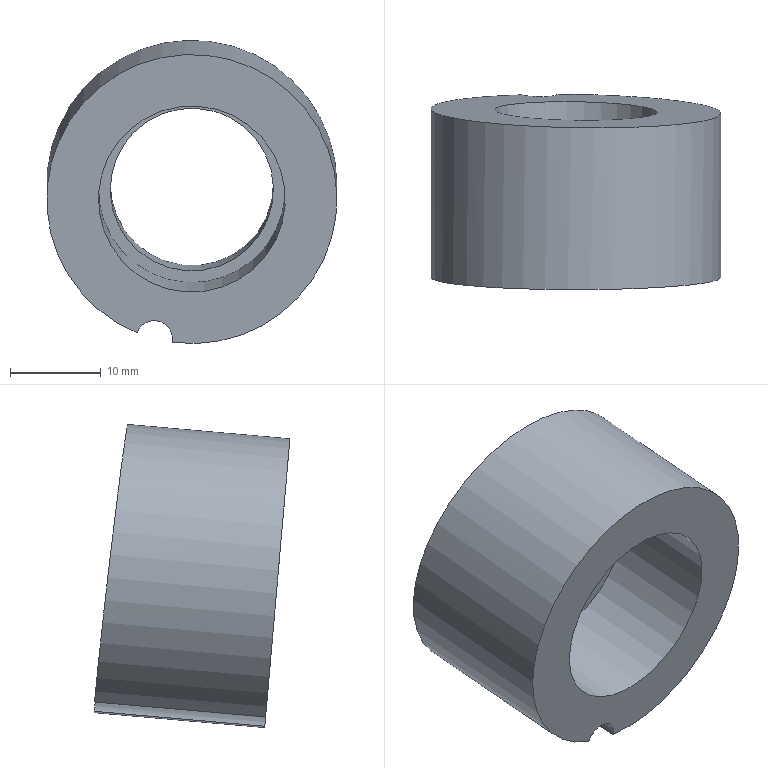Part | NX | features EKSD 32-20-18.00 2 | 1 solid | 7 faces | box 32 x 21.595 x 33.441 mm | volume 9053 mm3 | cylinder 4 | plane 3 | commonest cylinder face diameters 4 x1 18 x1 20.6 x1 32 x1
STEP:
#1=CARTESIAN_POINT('',(145.285,40.007,-46.316));
#2=VERTEX_POINT('',#1);
#3=CARTESIAN_POINT('',(141.429,39.917,-45.287));
#4=VERTEX_POINT('',#3);
#5=CARTESIAN_POINT('',(143.325,39.972,-45.922));
#6=DIRECTION('',(0.,-0.9962,-0.08716));
#7=DIRECTION('',(0.2588,-0.08419,0.9623));
#8=AXIS2_PLACEMENT_3D('',#5,#6,#7);
#9=CIRCLE('',#8,2.);
#10=EDGE_CURVE('',#2,#4,#9,.T.);
#11=ORIENTED_EDGE('',*,*,#10,.F.);
#12=CARTESIAN_POINT('',(147.466,38.625,-30.526));
#13=DIRECTION('',(0.,-0.9962,-0.08716));
#14=DIRECTION('',(0.2588,-0.08419,0.9623));
#15=AXIS2_PLACEMENT_3D('',#12,#13,#14);
#16=CIRCLE('',#15,16.);
#17=EDGE_CURVE('',#2,#4,#16,.T.);
#18=ORIENTED_EDGE('',*,*,#17,.T.);
#19=EDGE_LOOP('',(#11,#18));
#20=FACE_BOUND('',#19,.T.);
#21=CARTESIAN_POINT('',(144.8,39.492,-40.437));
#22=VERTEX_POINT('',#21);
#23=CARTESIAN_POINT('',(147.466,38.625,-30.526));
#24=DIRECTION('',(0.,0.9962,0.08716));
#25=DIRECTION('',(-0.2588,0.08419,-0.9623));
#26=AXIS2_PLACEMENT_3D('',#23,#24,#25);
#27=CIRCLE('',#26,10.3);
#28=EDGE_CURVE('',#22,#22,#27,.T.);
#29=ORIENTED_EDGE('',*,*,#28,.T.);
#30=EDGE_LOOP('',(#29));
#31=FACE_BOUND('',#30,.T.);
#32=CARTESIAN_POINT('',(147.466,38.625,-30.526));
#33=DIRECTION('',(0.,-0.9962,-0.08716));
#34=DIRECTION('',(-0.2588,0.08419,-0.9623));
#35=AXIS2_PLACEMENT_3D('',#32,#33,#34);
#36=PLANE('',#35);
#37=ADVANCED_FACE('',(#20,#31),#36,.T.);
#38=CARTESIAN_POINT('',(141.429,58.765,-43.638));
#39=VERTEX_POINT('',#38);
#40=CARTESIAN_POINT('',(145.285,58.826,-44.67));
#41=VERTEX_POINT('',#40);
#42=CARTESIAN_POINT('',(143.325,58.81,-44.274));
#43=DIRECTION('',(0.01549,0.9931,0.116));
#44=DIRECTION('',(0.4705,-0.1096,0.8755));
#45=AXIS2_PLACEMENT_3D('',#42,#43,#44);
#46=ELLIPSE('',#45,2.001,2.);
#47=EDGE_CURVE('',#39,#41,#46,.T.);
#48=ORIENTED_EDGE('',*,*,#47,.F.);
#49=CARTESIAN_POINT('',(147.466,56.952,-28.923));
#50=DIRECTION('',(0.01549,0.9931,0.116));
#51=DIRECTION('',(0.4705,-0.1096,0.8755));
#52=AXIS2_PLACEMENT_3D('',#49,#50,#51);
#53=ELLIPSE('',#52,16.009,16.);
#54=EDGE_CURVE('',#39,#41,#53,.T.);
#55=ORIENTED_EDGE('',*,*,#54,.T.);
#56=EDGE_LOOP('',(#48,#55));
#57=FACE_BOUND('',#56,.T.);
#58=CARTESIAN_POINT('',(151.703,55.965,-21.038));
#59=VERTEX_POINT('',#58);
#60=CARTESIAN_POINT('',(147.466,56.952,-28.923));
#61=DIRECTION('',(0.01549,0.9931,0.116));
#62=DIRECTION('',(0.4705,-0.1096,0.8755));
#63=AXIS2_PLACEMENT_3D('',#60,#61,#62);
#64=ELLIPSE('',#63,9.005,9.);
#65=EDGE_CURVE('',#59,#59,#64,.F.);
#66=ORIENTED_EDGE('',*,*,#65,.T.);
#67=EDGE_LOOP('',(#66));
#68=FACE_BOUND('',#67,.T.);
#69=CARTESIAN_POINT('',(159.246,62.921,-81.584));
#70=DIRECTION('',(0.01549,0.9931,0.116));
#71=DIRECTION('',(0.06594,-0.1168,0.991));
#72=AXIS2_PLACEMENT_3D('',#69,#70,#71);
#73=PLANE('',#72);
#74=ADVANCED_FACE('',(#57,#68),#73,.T.);
#75=CARTESIAN_POINT('',(141.429,49.879,-44.416));
#76=DIRECTION('',(0.,-0.9962,-0.08716));
#77=VECTOR('',#76,1000.);
#78=LINE('',#75,#77);
#79=EDGE_CURVE('',#39,#4,#78,.T.);
#80=ORIENTED_EDGE('',*,*,#79,.T.);
#81=ORIENTED_EDGE('',*,*,#17,.F.);
#82=CARTESIAN_POINT('',(145.285,49.969,-45.445));
#83=DIRECTION('',(0.,-0.9962,-0.08716));
#84=VECTOR('',#83,1000.);
#85=LINE('',#82,#84);
#86=EDGE_CURVE('',#2,#41,#85,.F.);
#87=ORIENTED_EDGE('',*,*,#86,.T.);
#88=ORIENTED_EDGE('',*,*,#54,.F.);
#89=EDGE_LOOP('',(#80,#81,#87,#88));
#90=FACE_BOUND('',#89,.T.);
#91=CARTESIAN_POINT('',(147.466,58.549,-28.783));
#92=DIRECTION('',(0.,-0.9962,-0.08716));
#93=DIRECTION('',(-0.2588,0.08419,-0.9623));
#94=AXIS2_PLACEMENT_3D('',#91,#92,#93);
#95=CYLINDRICAL_SURFACE('',#94,16.);
#96=ADVANCED_FACE('',(#90),#95,.T.);
#97=CARTESIAN_POINT('',(149.795,49.822,-20.82));
#98=VERTEX_POINT('',#97);
#99=CARTESIAN_POINT('',(147.466,50.58,-29.48));
#100=DIRECTION('',(0.,-0.9962,-0.08716));
#101=DIRECTION('',(0.2588,-0.08419,0.9623));
#102=AXIS2_PLACEMENT_3D('',#99,#100,#101);
#103=CIRCLE('',#102,9.);
#104=EDGE_CURVE('',#98,#98,#103,.F.);
#105=ORIENTED_EDGE('',*,*,#104,.F.);
#106=EDGE_LOOP('',(#105));
#107=FACE_BOUND('',#106,.T.);
#108=ORIENTED_EDGE('',*,*,#65,.F.);
#109=EDGE_LOOP('',(#108));
#110=FACE_BOUND('',#109,.T.);
#111=CARTESIAN_POINT('',(147.466,59.545,-28.696));
#112=DIRECTION('',(0.,-0.9962,-0.08716));
#113=DIRECTION('',(-0.2588,0.08419,-0.9623));
#114=AXIS2_PLACEMENT_3D('',#111,#112,#113);
#115=CYLINDRICAL_SURFACE('',#114,9.);
#116=ADVANCED_FACE('',(#107,#110),#115,.F.);
#117=CARTESIAN_POINT('',(144.8,51.447,-39.391));
#118=VERTEX_POINT('',#117);
#119=CARTESIAN_POINT('',(147.466,50.58,-29.48));
#120=DIRECTION('',(0.,0.9962,0.08716));
#121=DIRECTION('',(-0.2588,0.08419,-0.9623));
#122=AXIS2_PLACEMENT_3D('',#119,#120,#121);
#123=CIRCLE('',#122,10.3);
#124=EDGE_CURVE('',#118,#118,#123,.T.);
#125=ORIENTED_EDGE('',*,*,#124,.F.);
#126=EDGE_LOOP('',(#125));
#127=FACE_BOUND('',#126,.T.);
#128=ORIENTED_EDGE('',*,*,#104,.T.);
#129=EDGE_LOOP('',(#128));
#130=FACE_BOUND('',#129,.T.);
#131=CARTESIAN_POINT('',(147.466,50.58,-29.48));
#132=DIRECTION('',(0.,0.9962,0.08716));
#133=DIRECTION('',(0.2588,-0.08419,0.9623));
#134=AXIS2_PLACEMENT_3D('',#131,#132,#133);
#135=PLANE('',#134);
#136=ADVANCED_FACE('',(#127,#130),#135,.F.);
#137=ORIENTED_EDGE('',*,*,#28,.F.);
#138=EDGE_LOOP('',(#137));
#139=FACE_BOUND('',#138,.T.);
#140=ORIENTED_EDGE('',*,*,#124,.T.);
#141=EDGE_LOOP('',(#140));
#142=FACE_BOUND('',#141,.T.);
#143=CARTESIAN_POINT('',(147.466,50.58,-29.48));
#144=DIRECTION('',(0.,-0.9962,-0.08716));
#145=DIRECTION('',(-0.2588,0.08419,-0.9623));
#146=AXIS2_PLACEMENT_3D('',#143,#144,#145);
#147=CYLINDRICAL_SURFACE('',#146,10.3);
#148=ADVANCED_FACE('',(#139,#142),#147,.F.);
#149=ORIENTED_EDGE('',*,*,#79,.F.);
#150=ORIENTED_EDGE('',*,*,#47,.T.);
#151=ORIENTED_EDGE('',*,*,#86,.F.);
#152=ORIENTED_EDGE('',*,*,#10,.T.);
#153=EDGE_LOOP('',(#149,#150,#151,#152));
#154=FACE_BOUND('',#153,.T.);
#155=CARTESIAN_POINT('',(143.325,59.896,-44.179));
#156=DIRECTION('',(0.,-0.9962,-0.08716));
#157=DIRECTION('',(-0.2588,0.08419,-0.9623));
#158=AXIS2_PLACEMENT_3D('',#155,#156,#157);
#159=CYLINDRICAL_SURFACE('',#158,2.);
#160=ADVANCED_FACE('',(#154),#159,.F.);
#161=CLOSED_SHELL('',(#37,#74,#96,#116,#136,#148,#160));
#162=MANIFOLD_SOLID_BREP('',#161);
#163=(LENGTH_UNIT()NAMED_UNIT(*)SI_UNIT(.MILLI.,.METRE.));
#164=UNCERTAINTY_MEASURE_WITH_UNIT(LENGTH_MEASURE(0.00001),#163,'','');
#165=(NAMED_UNIT(*)PLANE_ANGLE_UNIT()SI_UNIT($,.RADIAN.));
#166=(NAMED_UNIT(*)SI_UNIT($,.STERADIAN.)SOLID_ANGLE_UNIT());
#167=(GEOMETRIC_REPRESENTATION_CONTEXT(3)GLOBAL_UNCERTAINTY_ASSIGNED_CONTEXT((#164))GLOBAL_UNIT_ASSIGNED_CONTEXT((#163,#165,#166))REPRESENTATION_CONTEXT('',''));
#168=ADVANCED_BREP_SHAPE_REPRESENTATION('',(#162),#167);